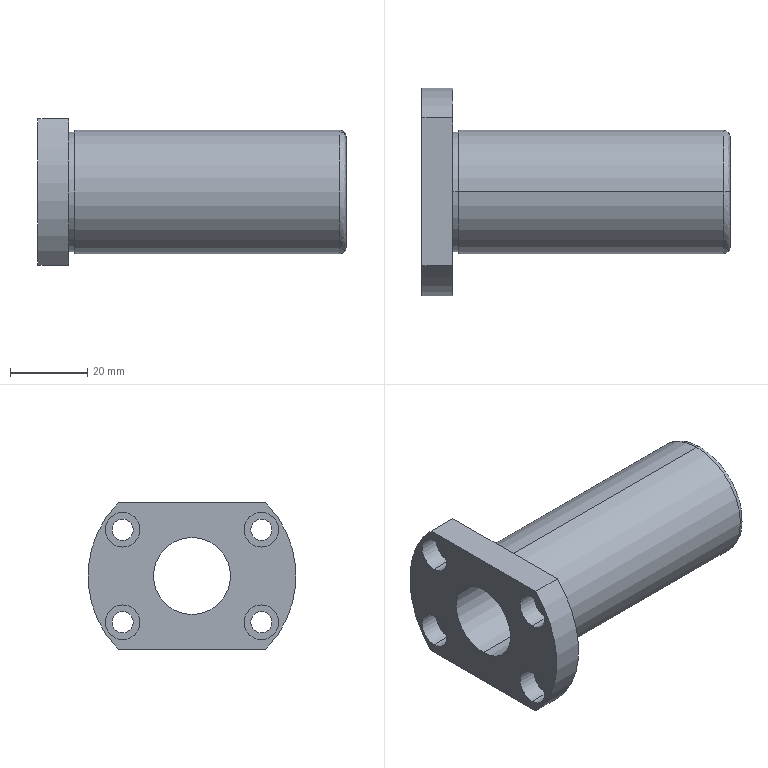Part | STEP file | lhfcwmf20_2_03 | 1 solid | 36 faces | box 80 x 54 x 38 mm | volume 46009 mm3 | cylinder 24 | plane 10 | spline 2 | commonest cylinder face diameters 5.5 x8 9 x8 20 x2 31 x2 32 x2 54 x2